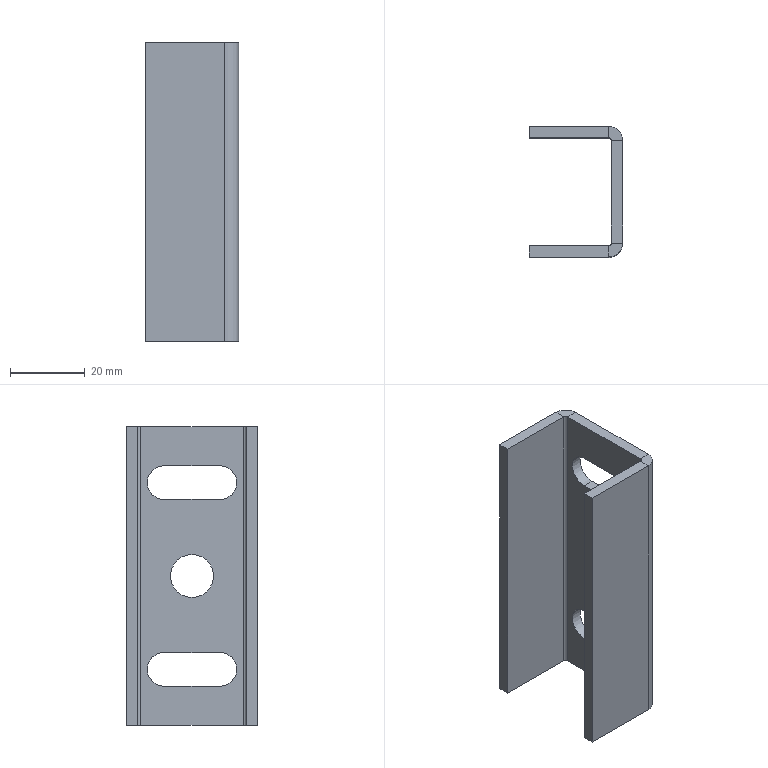Part | SolidWorks | features EdgeFlange 1, FlatPattern 1, SMBaseFlange 1, SheetMetal 1 | 1 solid | 32 faces | box 25 x 35 x 80 mm | volume 16996 mm3 | plane 22 | cylinder 10 | commonest cylinder face diameters 9 x4 1.473 x2 7.473 x2 11.5 x2
STEP:
#1=CARTESIAN_POINT('',(-3.,-17.5,-34.25));
#2=VERTEX_POINT('',#1);
#3=CARTESIAN_POINT('',(-3.,-17.5,-45.75));
#4=VERTEX_POINT('',#3);
#5=CARTESIAN_POINT('',(-3.,-17.5,-40.));
#6=DIRECTION('',(1.,0.,0.));
#7=DIRECTION('',(0.,0.,-1.));
#8=AXIS2_PLACEMENT_3D('',#5,#6,#7);
#9=CIRCLE('',#8,5.75);
#10=EDGE_CURVE('',#2,#4,#9,.T.);
#11=ORIENTED_EDGE('',*,*,#10,.F.);
#12=CARTESIAN_POINT('',(0.,-17.5,-34.25));
#13=VERTEX_POINT('',#12);
#14=CARTESIAN_POINT('',(-3.,-17.5,-34.25));
#15=DIRECTION('',(1.,0.,0.));
#16=VECTOR('',#15,1000.);
#17=LINE('',#14,#16);
#18=EDGE_CURVE('',#2,#13,#17,.T.);
#19=ORIENTED_EDGE('',*,*,#18,.T.);
#20=CARTESIAN_POINT('',(0.,-17.5,-45.75));
#21=VERTEX_POINT('',#20);
#22=CARTESIAN_POINT('',(0.,-17.5,-40.));
#23=DIRECTION('',(1.,0.,0.));
#24=DIRECTION('',(0.,0.,-1.));
#25=AXIS2_PLACEMENT_3D('',#22,#23,#24);
#26=CIRCLE('',#25,5.75);
#27=EDGE_CURVE('',#13,#21,#26,.T.);
#28=ORIENTED_EDGE('',*,*,#27,.T.);
#29=CARTESIAN_POINT('',(-3.,-17.5,-45.75));
#30=DIRECTION('',(1.,0.,0.));
#31=VECTOR('',#30,1000.);
#32=LINE('',#29,#31);
#33=EDGE_CURVE('',#4,#21,#32,.T.);
#34=ORIENTED_EDGE('',*,*,#33,.F.);
#35=EDGE_LOOP('',(#11,#19,#28,#34));
#36=FACE_OUTER_BOUND('',#35,.T.);
#37=CARTESIAN_POINT('',(-3.,-17.5,-40.));
#38=DIRECTION('',(1.,0.,0.));
#39=DIRECTION('',(0.,0.,-1.));
#40=AXIS2_PLACEMENT_3D('',#37,#38,#39);
#41=CYLINDRICAL_SURFACE('',#40,5.75);
#42=ADVANCED_FACE('',(#36),#41,.F.);
#43=CARTESIAN_POINT('',(-3.,-25.,-69.5));
#44=VERTEX_POINT('',#43);
#45=CARTESIAN_POINT('',(-3.,-10.,-69.5));
#46=VERTEX_POINT('',#45);
#47=CARTESIAN_POINT('',(-3.,-10.,-69.5));
#48=DIRECTION('',(0.,1.,0.));
#49=VECTOR('',#48,1000.);
#50=LINE('',#47,#49);
#51=EDGE_CURVE('',#44,#46,#50,.T.);
#52=ORIENTED_EDGE('',*,*,#51,.T.);
#53=CARTESIAN_POINT('',(-3.,-10.,-60.5));
#54=VERTEX_POINT('',#53);
#55=CARTESIAN_POINT('',(-3.,-10.,-65.));
#56=DIRECTION('',(1.,0.,0.));
#57=DIRECTION('',(0.,0.,-1.));
#58=AXIS2_PLACEMENT_3D('',#55,#56,#57);
#59=CIRCLE('',#58,4.5);
#60=EDGE_CURVE('',#46,#54,#59,.T.);
#61=ORIENTED_EDGE('',*,*,#60,.T.);
#62=CARTESIAN_POINT('',(-3.,-25.,-60.5));
#63=VERTEX_POINT('',#62);
#64=CARTESIAN_POINT('',(-3.,-10.,-60.5));
#65=DIRECTION('',(0.,-1.,0.));
#66=VECTOR('',#65,1000.);
#67=LINE('',#64,#66);
#68=EDGE_CURVE('',#54,#63,#67,.T.);
#69=ORIENTED_EDGE('',*,*,#68,.T.);
#70=CARTESIAN_POINT('',(-3.,-25.,-65.));
#71=DIRECTION('',(1.,0.,0.));
#72=DIRECTION('',(0.,0.,-1.));
#73=AXIS2_PLACEMENT_3D('',#70,#71,#72);
#74=CIRCLE('',#73,4.5);
#75=EDGE_CURVE('',#63,#44,#74,.T.);
#76=ORIENTED_EDGE('',*,*,#75,.T.);
#77=EDGE_LOOP('',(#52,#61,#69,#76));
#78=FACE_BOUND('',#77,.T.);
#79=CARTESIAN_POINT('',(-3.,-25.,-19.5));
#80=VERTEX_POINT('',#79);
#81=CARTESIAN_POINT('',(-3.,-10.,-19.5));
#82=VERTEX_POINT('',#81);
#83=CARTESIAN_POINT('',(-3.,-10.,-19.5));
#84=DIRECTION('',(0.,1.,0.));
#85=VECTOR('',#84,1000.);
#86=LINE('',#83,#85);
#87=EDGE_CURVE('',#80,#82,#86,.T.);
#88=ORIENTED_EDGE('',*,*,#87,.T.);
#89=CARTESIAN_POINT('',(-3.,-10.,-10.5));
#90=VERTEX_POINT('',#89);
#91=CARTESIAN_POINT('',(-3.,-10.,-15.));
#92=DIRECTION('',(1.,0.,0.));
#93=DIRECTION('',(0.,0.,-1.));
#94=AXIS2_PLACEMENT_3D('',#91,#92,#93);
#95=CIRCLE('',#94,4.5);
#96=EDGE_CURVE('',#82,#90,#95,.T.);
#97=ORIENTED_EDGE('',*,*,#96,.T.);
#98=CARTESIAN_POINT('',(-3.,-25.,-10.5));
#99=VERTEX_POINT('',#98);
#100=CARTESIAN_POINT('',(-3.,-10.,-10.5));
#101=DIRECTION('',(0.,-1.,0.));
#102=VECTOR('',#101,1000.);
#103=LINE('',#100,#102);
#104=EDGE_CURVE('',#90,#99,#103,.T.);
#105=ORIENTED_EDGE('',*,*,#104,.T.);
#106=CARTESIAN_POINT('',(-3.,-25.,-15.));
#107=DIRECTION('',(1.,0.,0.));
#108=DIRECTION('',(0.,0.,-1.));
#109=AXIS2_PLACEMENT_3D('',#106,#107,#108);
#110=CIRCLE('',#109,4.5);
#111=EDGE_CURVE('',#99,#80,#110,.T.);
#112=ORIENTED_EDGE('',*,*,#111,.T.);
#113=EDGE_LOOP('',(#88,#97,#105,#112));
#114=FACE_BOUND('',#113,.T.);
#115=CARTESIAN_POINT('',(-3.,-17.5,-40.));
#116=DIRECTION('',(1.,0.,0.));
#117=DIRECTION('',(0.,0.,-1.));
#118=AXIS2_PLACEMENT_3D('',#115,#116,#117);
#119=CIRCLE('',#118,5.75);
#120=EDGE_CURVE('',#4,#2,#119,.T.);
#121=ORIENTED_EDGE('',*,*,#120,.T.);
#122=ORIENTED_EDGE('',*,*,#10,.T.);
#123=EDGE_LOOP('',(#121,#122));
#124=FACE_BOUND('',#123,.T.);
#125=CARTESIAN_POINT('',(-3.,-31.263,0.));
#126=VERTEX_POINT('',#125);
#127=CARTESIAN_POINT('',(-3.,-31.263,-80.));
#128=VERTEX_POINT('',#127);
#129=CARTESIAN_POINT('',(-3.,-31.263,0.));
#130=DIRECTION('',(0.,0.,-1.));
#131=VECTOR('',#130,1000.);
#132=LINE('',#129,#131);
#133=EDGE_CURVE('',#126,#128,#132,.T.);
#134=ORIENTED_EDGE('',*,*,#133,.F.);
#135=CARTESIAN_POINT('',(-3.,-3.737,0.));
#136=VERTEX_POINT('',#135);
#137=CARTESIAN_POINT('',(-3.,0.,0.));
#138=DIRECTION('',(0.,-1.,0.));
#139=VECTOR('',#138,1000.);
#140=LINE('',#137,#139);
#141=EDGE_CURVE('',#136,#126,#140,.T.);
#142=ORIENTED_EDGE('',*,*,#141,.F.);
#143=CARTESIAN_POINT('',(-3.,-3.737,-80.));
#144=VERTEX_POINT('',#143);
#145=CARTESIAN_POINT('',(-3.,-3.737,-80.));
#146=DIRECTION('',(0.,0.,1.));
#147=VECTOR('',#146,1000.);
#148=LINE('',#145,#147);
#149=EDGE_CURVE('',#144,#136,#148,.T.);
#150=ORIENTED_EDGE('',*,*,#149,.F.);
#151=CARTESIAN_POINT('',(-3.,0.,-80.));
#152=DIRECTION('',(0.,1.,0.));
#153=VECTOR('',#152,1000.);
#154=LINE('',#151,#153);
#155=EDGE_CURVE('',#128,#144,#154,.T.);
#156=ORIENTED_EDGE('',*,*,#155,.F.);
#157=EDGE_LOOP('',(#134,#142,#150,#156));
#158=FACE_OUTER_BOUND('',#157,.T.);
#159=CARTESIAN_POINT('',(-3.,0.,0.));
#160=DIRECTION('',(1.,0.,0.));
#161=DIRECTION('',(0.,0.,-1.));
#162=AXIS2_PLACEMENT_3D('',#159,#160,#161);
#163=PLANE('',#162);
#164=ADVANCED_FACE('',(#78,#114,#124,#158),#163,.F.);
#165=CARTESIAN_POINT('',(0.,-10.,-69.5));
#166=VERTEX_POINT('',#165);
#167=CARTESIAN_POINT('',(0.,-10.,-60.5));
#168=VERTEX_POINT('',#167);
#169=CARTESIAN_POINT('',(0.,-10.,-65.));
#170=DIRECTION('',(1.,0.,0.));
#171=DIRECTION('',(0.,0.,-1.));
#172=AXIS2_PLACEMENT_3D('',#169,#170,#171);
#173=CIRCLE('',#172,4.5);
#174=EDGE_CURVE('',#166,#168,#173,.T.);
#175=ORIENTED_EDGE('',*,*,#174,.F.);
#176=CARTESIAN_POINT('',(0.,-25.,-69.5));
#177=VERTEX_POINT('',#176);
#178=CARTESIAN_POINT('',(0.,-10.,-69.5));
#179=DIRECTION('',(0.,1.,0.));
#180=VECTOR('',#179,1000.);
#181=LINE('',#178,#180);
#182=EDGE_CURVE('',#177,#166,#181,.T.);
#183=ORIENTED_EDGE('',*,*,#182,.F.);
#184=CARTESIAN_POINT('',(0.,-25.,-60.5));
#185=VERTEX_POINT('',#184);
#186=CARTESIAN_POINT('',(0.,-25.,-65.));
#187=DIRECTION('',(1.,0.,0.));
#188=DIRECTION('',(0.,0.,-1.));
#189=AXIS2_PLACEMENT_3D('',#186,#187,#188);
#190=CIRCLE('',#189,4.5);
#191=EDGE_CURVE('',#185,#177,#190,.T.);
#192=ORIENTED_EDGE('',*,*,#191,.F.);
#193=CARTESIAN_POINT('',(0.,-10.,-60.5));
#194=DIRECTION('',(0.,-1.,0.));
#195=VECTOR('',#194,1000.);
#196=LINE('',#193,#195);
#197=EDGE_CURVE('',#168,#185,#196,.T.);
#198=ORIENTED_EDGE('',*,*,#197,.F.);
#199=EDGE_LOOP('',(#175,#183,#192,#198));
#200=FACE_BOUND('',#199,.T.);
#201=CARTESIAN_POINT('',(0.,-10.,-19.5));
#202=VERTEX_POINT('',#201);
#203=CARTESIAN_POINT('',(0.,-10.,-10.5));
#204=VERTEX_POINT('',#203);
#205=CARTESIAN_POINT('',(0.,-10.,-15.));
#206=DIRECTION('',(1.,0.,0.));
#207=DIRECTION('',(0.,0.,-1.));
#208=AXIS2_PLACEMENT_3D('',#205,#206,#207);
#209=CIRCLE('',#208,4.5);
#210=EDGE_CURVE('',#202,#204,#209,.T.);
#211=ORIENTED_EDGE('',*,*,#210,.F.);
#212=CARTESIAN_POINT('',(0.,-25.,-19.5));
#213=VERTEX_POINT('',#212);
#214=CARTESIAN_POINT('',(0.,-10.,-19.5));
#215=DIRECTION('',(0.,1.,0.));
#216=VECTOR('',#215,1000.);
#217=LINE('',#214,#216);
#218=EDGE_CURVE('',#213,#202,#217,.T.);
#219=ORIENTED_EDGE('',*,*,#218,.F.);
#220=CARTESIAN_POINT('',(0.,-25.,-10.5));
#221=VERTEX_POINT('',#220);
#222=CARTESIAN_POINT('',(0.,-25.,-15.));
#223=DIRECTION('',(1.,0.,0.));
#224=DIRECTION('',(0.,0.,-1.));
#225=AXIS2_PLACEMENT_3D('',#222,#223,#224);
#226=CIRCLE('',#225,4.5);
#227=EDGE_CURVE('',#221,#213,#226,.T.);
#228=ORIENTED_EDGE('',*,*,#227,.F.);
#229=CARTESIAN_POINT('',(0.,-10.,-10.5));
#230=DIRECTION('',(0.,-1.,0.));
#231=VECTOR('',#230,1000.);
#232=LINE('',#229,#231);
#233=EDGE_CURVE('',#204,#221,#232,.T.);
#234=ORIENTED_EDGE('',*,*,#233,.F.);
#235=EDGE_LOOP('',(#211,#219,#228,#234));
#236=FACE_BOUND('',#235,.T.);
#237=CARTESIAN_POINT('',(0.,-17.5,-40.));
#238=DIRECTION('',(1.,0.,0.));
#239=DIRECTION('',(0.,0.,-1.));
#240=AXIS2_PLACEMENT_3D('',#237,#238,#239);
#241=CIRCLE('',#240,5.75);
#242=EDGE_CURVE('',#21,#13,#241,.T.);
#243=ORIENTED_EDGE('',*,*,#242,.F.);
#244=ORIENTED_EDGE('',*,*,#27,.F.);
#245=EDGE_LOOP('',(#243,#244));
#246=FACE_BOUND('',#245,.T.);
#247=CARTESIAN_POINT('',(0.,-3.737,0.));
#248=VERTEX_POINT('',#247);
#249=CARTESIAN_POINT('',(0.,-31.263,0.));
#250=VERTEX_POINT('',#249);
#251=CARTESIAN_POINT('',(0.,0.,0.));
#252=DIRECTION('',(0.,-1.,0.));
#253=VECTOR('',#252,1000.);
#254=LINE('',#251,#253);
#255=EDGE_CURVE('',#248,#250,#254,.T.);
#256=ORIENTED_EDGE('',*,*,#255,.T.);
#257=CARTESIAN_POINT('',(0.,-31.263,-80.));
#258=VERTEX_POINT('',#257);
#259=CARTESIAN_POINT('',(0.,-31.263,0.));
#260=DIRECTION('',(0.,0.,-1.));
#261=VECTOR('',#260,1000.);
#262=LINE('',#259,#261);
#263=EDGE_CURVE('',#250,#258,#262,.T.);
#264=ORIENTED_EDGE('',*,*,#263,.T.);
#265=CARTESIAN_POINT('',(0.,-3.737,-80.));
#266=VERTEX_POINT('',#265);
#267=CARTESIAN_POINT('',(0.,0.,-80.));
#268=DIRECTION('',(0.,1.,0.));
#269=VECTOR('',#268,1000.);
#270=LINE('',#267,#269);
#271=EDGE_CURVE('',#258,#266,#270,.T.);
#272=ORIENTED_EDGE('',*,*,#271,.T.);
#273=CARTESIAN_POINT('',(0.,-3.737,-80.));
#274=DIRECTION('',(0.,0.,1.));
#275=VECTOR('',#274,1000.);
#276=LINE('',#273,#275);
#277=EDGE_CURVE('',#266,#248,#276,.T.);
#278=ORIENTED_EDGE('',*,*,#277,.T.);
#279=EDGE_LOOP('',(#256,#264,#272,#278));
#280=FACE_OUTER_BOUND('',#279,.T.);
#281=CARTESIAN_POINT('',(0.,0.,0.));
#282=DIRECTION('',(1.,0.,0.));
#283=DIRECTION('',(0.,0.,-1.));
#284=AXIS2_PLACEMENT_3D('',#281,#282,#283);
#285=PLANE('',#284);
#286=ADVANCED_FACE('',(#200,#236,#246,#280),#285,.T.);
#287=ORIENTED_EDGE('',*,*,#141,.T.);
#288=CARTESIAN_POINT('',(-3.,-31.263,0.));
#289=DIRECTION('',(1.,0.,0.));
#290=VECTOR('',#289,1000.);
#291=LINE('',#288,#290);
#292=EDGE_CURVE('',#126,#250,#291,.T.);
#293=ORIENTED_EDGE('',*,*,#292,.T.);
#294=ORIENTED_EDGE('',*,*,#255,.F.);
#295=CARTESIAN_POINT('',(-3.,-3.737,0.));
#296=DIRECTION('',(1.,0.,0.));
#297=VECTOR('',#296,1000.);
#298=LINE('',#295,#297);
#299=EDGE_CURVE('',#136,#248,#298,.T.);
#300=ORIENTED_EDGE('',*,*,#299,.F.);
#301=EDGE_LOOP('',(#287,#293,#294,#300));
#302=FACE_OUTER_BOUND('',#301,.T.);
#303=CARTESIAN_POINT('',(-3.,0.,0.));
#304=DIRECTION('',(0.,0.,1.));
#305=DIRECTION('',(0.,-1.,0.));
#306=AXIS2_PLACEMENT_3D('',#303,#304,#305);
#307=PLANE('',#306);
#308=ADVANCED_FACE('',(#302),#307,.T.);
#309=CARTESIAN_POINT('',(-3.,-31.263,-80.));
#310=DIRECTION('',(1.,0.,0.));
#311=VECTOR('',#310,1000.);
#312=LINE('',#309,#311);
#313=EDGE_CURVE('',#128,#258,#312,.T.);
#314=ORIENTED_EDGE('',*,*,#313,.F.);
#315=ORIENTED_EDGE('',*,*,#155,.T.);
#316=CARTESIAN_POINT('',(-3.,-3.737,-80.));
#317=DIRECTION('',(1.,0.,0.));
#318=VECTOR('',#317,1000.);
#319=LINE('',#316,#318);
#320=EDGE_CURVE('',#144,#266,#319,.T.);
#321=ORIENTED_EDGE('',*,*,#320,.T.);
#322=ORIENTED_EDGE('',*,*,#271,.F.);
#323=EDGE_LOOP('',(#314,#315,#321,#322));
#324=FACE_OUTER_BOUND('',#323,.T.);
#325=CARTESIAN_POINT('',(-3.,0.,-80.));
#326=DIRECTION('',(0.,0.,-1.));
#327=DIRECTION('',(-1.,0.,0.));
#328=AXIS2_PLACEMENT_3D('',#325,#326,#327);
#329=PLANE('',#328);
#330=ADVANCED_FACE('',(#324),#329,.T.);
#331=ORIENTED_EDGE('',*,*,#18,.F.);
#332=ORIENTED_EDGE('',*,*,#120,.F.);
#333=ORIENTED_EDGE('',*,*,#33,.T.);
#334=ORIENTED_EDGE('',*,*,#242,.T.);
#335=EDGE_LOOP('',(#331,#332,#333,#334));
#336=FACE_OUTER_BOUND('',#335,.T.);
#337=CARTESIAN_POINT('',(-3.,-17.5,-40.));
#338=DIRECTION('',(1.,0.,0.));
#339=DIRECTION('',(0.,0.,-1.));
#340=AXIS2_PLACEMENT_3D('',#337,#338,#339);
#341=CYLINDRICAL_SURFACE('',#340,5.75);
#342=ADVANCED_FACE('',(#336),#341,.F.);
#343=ORIENTED_EDGE('',*,*,#210,.T.);
#344=CARTESIAN_POINT('',(-3.,-10.,-10.5));
#345=DIRECTION('',(1.,0.,0.));
#346=VECTOR('',#345,1000.);
#347=LINE('',#344,#346);
#348=EDGE_CURVE('',#90,#204,#347,.T.);
#349=ORIENTED_EDGE('',*,*,#348,.F.);
#350=ORIENTED_EDGE('',*,*,#96,.F.);
#351=CARTESIAN_POINT('',(-3.,-10.,-19.5));
#352=DIRECTION('',(1.,0.,0.));
#353=VECTOR('',#352,1000.);
#354=LINE('',#351,#353);
#355=EDGE_CURVE('',#82,#202,#354,.T.);
#356=ORIENTED_EDGE('',*,*,#355,.T.);
#357=EDGE_LOOP('',(#343,#349,#350,#356));
#358=FACE_OUTER_BOUND('',#357,.T.);
#359=CARTESIAN_POINT('',(-3.,-10.,-15.));
#360=DIRECTION('',(1.,0.,0.));
#361=DIRECTION('',(0.,0.,-1.));
#362=AXIS2_PLACEMENT_3D('',#359,#360,#361);
#363=CYLINDRICAL_SURFACE('',#362,4.5);
#364=ADVANCED_FACE('',(#358),#363,.F.);
#365=ORIENTED_EDGE('',*,*,#218,.T.);
#366=ORIENTED_EDGE('',*,*,#355,.F.);
#367=ORIENTED_EDGE('',*,*,#87,.F.);
#368=CARTESIAN_POINT('',(-3.,-25.,-19.5));
#369=DIRECTION('',(1.,0.,0.));
#370=VECTOR('',#369,1000.);
#371=LINE('',#368,#370);
#372=EDGE_CURVE('',#80,#213,#371,.T.);
#373=ORIENTED_EDGE('',*,*,#372,.T.);
#374=EDGE_LOOP('',(#365,#366,#367,#373));
#375=FACE_OUTER_BOUND('',#374,.T.);
#376=CARTESIAN_POINT('',(-3.,-10.,-19.5));
#377=DIRECTION('',(0.,0.,-1.));
#378=DIRECTION('',(0.,1.,0.));
#379=AXIS2_PLACEMENT_3D('',#376,#377,#378);
#380=PLANE('',#379);
#381=ADVANCED_FACE('',(#375),#380,.F.);
#382=ORIENTED_EDGE('',*,*,#227,.T.);
#383=ORIENTED_EDGE('',*,*,#372,.F.);
#384=ORIENTED_EDGE('',*,*,#111,.F.);
#385=CARTESIAN_POINT('',(-3.,-25.,-10.5));
#386=DIRECTION('',(1.,0.,0.));
#387=VECTOR('',#386,1000.);
#388=LINE('',#385,#387);
#389=EDGE_CURVE('',#99,#221,#388,.T.);
#390=ORIENTED_EDGE('',*,*,#389,.T.);
#391=EDGE_LOOP('',(#382,#383,#384,#390));
#392=FACE_OUTER_BOUND('',#391,.T.);
#393=CARTESIAN_POINT('',(-3.,-25.,-15.));
#394=DIRECTION('',(1.,0.,0.));
#395=DIRECTION('',(0.,0.,-1.));
#396=AXIS2_PLACEMENT_3D('',#393,#394,#395);
#397=CYLINDRICAL_SURFACE('',#396,4.5);
#398=ADVANCED_FACE('',(#392),#397,.F.);
#399=ORIENTED_EDGE('',*,*,#233,.T.);
#400=ORIENTED_EDGE('',*,*,#389,.F.);
#401=ORIENTED_EDGE('',*,*,#104,.F.);
#402=ORIENTED_EDGE('',*,*,#348,.T.);
#403=EDGE_LOOP('',(#399,#400,#401,#402));
#404=FACE_OUTER_BOUND('',#403,.T.);
#405=CARTESIAN_POINT('',(-3.,-10.,-10.5));
#406=DIRECTION('',(0.,0.,1.));
#407=DIRECTION('',(0.,-1.,0.));
#408=AXIS2_PLACEMENT_3D('',#405,#406,#407);
#409=PLANE('',#408);
#410=ADVANCED_FACE('',(#404),#409,.F.);
#411=ORIENTED_EDGE('',*,*,#174,.T.);
#412=CARTESIAN_POINT('',(-3.,-10.,-60.5));
#413=DIRECTION('',(1.,0.,0.));
#414=VECTOR('',#413,1000.);
#415=LINE('',#412,#414);
#416=EDGE_CURVE('',#54,#168,#415,.T.);
#417=ORIENTED_EDGE('',*,*,#416,.F.);
#418=ORIENTED_EDGE('',*,*,#60,.F.);
#419=CARTESIAN_POINT('',(-3.,-10.,-69.5));
#420=DIRECTION('',(1.,0.,0.));
#421=VECTOR('',#420,1000.);
#422=LINE('',#419,#421);
#423=EDGE_CURVE('',#46,#166,#422,.T.);
#424=ORIENTED_EDGE('',*,*,#423,.T.);
#425=EDGE_LOOP('',(#411,#417,#418,#424));
#426=FACE_OUTER_BOUND('',#425,.T.);
#427=CARTESIAN_POINT('',(-3.,-10.,-65.));
#428=DIRECTION('',(1.,0.,0.));
#429=DIRECTION('',(0.,0.,-1.));
#430=AXIS2_PLACEMENT_3D('',#427,#428,#429);
#431=CYLINDRICAL_SURFACE('',#430,4.5);
#432=ADVANCED_FACE('',(#426),#431,.F.);
#433=ORIENTED_EDGE('',*,*,#182,.T.);
#434=ORIENTED_EDGE('',*,*,#423,.F.);
#435=ORIENTED_EDGE('',*,*,#51,.F.);
#436=CARTESIAN_POINT('',(-3.,-25.,-69.5));
#437=DIRECTION('',(1.,0.,0.));
#438=VECTOR('',#437,1000.);
#439=LINE('',#436,#438);
#440=EDGE_CURVE('',#44,#177,#439,.T.);
#441=ORIENTED_EDGE('',*,*,#440,.T.);
#442=EDGE_LOOP('',(#433,#434,#435,#441));
#443=FACE_OUTER_BOUND('',#442,.T.);
#444=CARTESIAN_POINT('',(-3.,-10.,-69.5));
#445=DIRECTION('',(0.,0.,-1.));
#446=DIRECTION('',(0.,1.,0.));
#447=AXIS2_PLACEMENT_3D('',#444,#445,#446);
#448=PLANE('',#447);
#449=ADVANCED_FACE('',(#443),#448,.F.);
#450=ORIENTED_EDGE('',*,*,#191,.T.);
#451=ORIENTED_EDGE('',*,*,#440,.F.);
#452=ORIENTED_EDGE('',*,*,#75,.F.);
#453=CARTESIAN_POINT('',(-3.,-25.,-60.5));
#454=DIRECTION('',(1.,0.,0.));
#455=VECTOR('',#454,1000.);
#456=LINE('',#453,#455);
#457=EDGE_CURVE('',#63,#185,#456,.T.);
#458=ORIENTED_EDGE('',*,*,#457,.T.);
#459=EDGE_LOOP('',(#450,#451,#452,#458));
#460=FACE_OUTER_BOUND('',#459,.T.);
#461=CARTESIAN_POINT('',(-3.,-25.,-65.));
#462=DIRECTION('',(1.,0.,0.));
#463=DIRECTION('',(0.,0.,-1.));
#464=AXIS2_PLACEMENT_3D('',#461,#462,#463);
#465=CYLINDRICAL_SURFACE('',#464,4.5);
#466=ADVANCED_FACE('',(#460),#465,.F.);
#467=ORIENTED_EDGE('',*,*,#197,.T.);
#468=ORIENTED_EDGE('',*,*,#457,.F.);
#469=ORIENTED_EDGE('',*,*,#68,.F.);
#470=ORIENTED_EDGE('',*,*,#416,.T.);
#471=EDGE_LOOP('',(#467,#468,#469,#470));
#472=FACE_OUTER_BOUND('',#471,.T.);
#473=CARTESIAN_POINT('',(-3.,-10.,-60.5));
#474=DIRECTION('',(0.,0.,1.));
#475=DIRECTION('',(0.,-1.,0.));
#476=AXIS2_PLACEMENT_3D('',#473,#474,#475);
#477=PLANE('',#476);
#478=ADVANCED_FACE('',(#472),#477,.F.);
#479=CARTESIAN_POINT('',(-3.737,-3.,0.));
#480=VERTEX_POINT('',#479);
#481=CARTESIAN_POINT('',(-3.737,0.,0.));
#482=VERTEX_POINT('',#481);
#483=CARTESIAN_POINT('',(-3.737,0.,0.));
#484=DIRECTION('',(0.,1.,0.));
#485=VECTOR('',#484,1000.);
#486=LINE('',#483,#485);
#487=EDGE_CURVE('',#480,#482,#486,.T.);
#488=ORIENTED_EDGE('',*,*,#487,.F.);
#489=CARTESIAN_POINT('',(-3.737,-3.737,0.));
#490=DIRECTION('',(0.,0.,1.));
#491=DIRECTION('',(-1.,0.,0.));
#492=AXIS2_PLACEMENT_3D('',#489,#490,#491);
#493=CIRCLE('',#492,0.7366);
#494=EDGE_CURVE('',#136,#480,#493,.T.);
#495=ORIENTED_EDGE('',*,*,#494,.F.);
#496=ORIENTED_EDGE('',*,*,#299,.T.);
#497=CARTESIAN_POINT('',(-3.737,-3.737,0.));
#498=DIRECTION('',(0.,0.,1.));
#499=DIRECTION('',(-1.,0.,0.));
#500=AXIS2_PLACEMENT_3D('',#497,#498,#499);
#501=CIRCLE('',#500,3.737);
#502=EDGE_CURVE('',#248,#482,#501,.T.);
#503=ORIENTED_EDGE('',*,*,#502,.T.);
#504=EDGE_LOOP('',(#488,#495,#496,#503));
#505=FACE_OUTER_BOUND('',#504,.T.);
#506=CARTESIAN_POINT('',(-3.737,-3.737,0.));
#507=DIRECTION('',(0.,0.,1.));
#508=DIRECTION('',(1.,0.,0.));
#509=AXIS2_PLACEMENT_3D('',#506,#507,#508);
#510=PLANE('',#509);
#511=ADVANCED_FACE('',(#505),#510,.T.);
#512=CARTESIAN_POINT('',(-3.737,-3.,-80.));
#513=VERTEX_POINT('',#512);
#514=CARTESIAN_POINT('',(-3.737,-3.737,-80.));
#515=DIRECTION('',(0.,0.,-1.));
#516=DIRECTION('',(-1.,0.,0.));
#517=AXIS2_PLACEMENT_3D('',#514,#515,#516);
#518=CIRCLE('',#517,0.7366);
#519=EDGE_CURVE('',#513,#144,#518,.T.);
#520=ORIENTED_EDGE('',*,*,#519,.F.);
#521=CARTESIAN_POINT('',(-3.737,0.,-80.));
#522=VERTEX_POINT('',#521);
#523=CARTESIAN_POINT('',(-3.737,-3.,-80.));
#524=DIRECTION('',(0.,1.,0.));
#525=VECTOR('',#524,1000.);
#526=LINE('',#523,#525);
#527=EDGE_CURVE('',#513,#522,#526,.T.);
#528=ORIENTED_EDGE('',*,*,#527,.T.);
#529=CARTESIAN_POINT('',(-3.737,-3.737,-80.));
#530=DIRECTION('',(0.,0.,-1.));
#531=DIRECTION('',(-1.,0.,0.));
#532=AXIS2_PLACEMENT_3D('',#529,#530,#531);
#533=CIRCLE('',#532,3.737);
#534=EDGE_CURVE('',#522,#266,#533,.T.);
#535=ORIENTED_EDGE('',*,*,#534,.T.);
#536=ORIENTED_EDGE('',*,*,#320,.F.);
#537=EDGE_LOOP('',(#520,#528,#535,#536));
#538=FACE_OUTER_BOUND('',#537,.T.);
#539=CARTESIAN_POINT('',(-3.737,-3.737,-80.));
#540=DIRECTION('',(0.,0.,1.));
#541=DIRECTION('',(1.,0.,0.));
#542=AXIS2_PLACEMENT_3D('',#539,#540,#541);
#543=PLANE('',#542);
#544=ADVANCED_FACE('',(#538),#543,.F.);
#545=ORIENTED_EDGE('',*,*,#277,.F.);
#546=ORIENTED_EDGE('',*,*,#534,.F.);
#547=CARTESIAN_POINT('',(-3.737,0.,0.));
#548=DIRECTION('',(0.,0.,1.));
#549=VECTOR('',#548,1000.);
#550=LINE('',#547,#549);
#551=EDGE_CURVE('',#522,#482,#550,.T.);
#552=ORIENTED_EDGE('',*,*,#551,.T.);
#553=ORIENTED_EDGE('',*,*,#502,.F.);
#554=EDGE_LOOP('',(#545,#546,#552,#553));
#555=FACE_OUTER_BOUND('',#554,.T.);
#556=CARTESIAN_POINT('',(-3.737,-3.737,-80.));
#557=DIRECTION('',(0.,0.,-1.));
#558=DIRECTION('',(0.,1.,0.));
#559=AXIS2_PLACEMENT_3D('',#556,#557,#558);
#560=CYLINDRICAL_SURFACE('',#559,3.737);
#561=ADVANCED_FACE('',(#555),#560,.T.);
#562=ORIENTED_EDGE('',*,*,#149,.T.);
#563=ORIENTED_EDGE('',*,*,#494,.T.);
#564=CARTESIAN_POINT('',(-3.737,-3.,0.));
#565=DIRECTION('',(0.,0.,-1.));
#566=VECTOR('',#565,1000.);
#567=LINE('',#564,#566);
#568=EDGE_CURVE('',#480,#513,#567,.T.);
#569=ORIENTED_EDGE('',*,*,#568,.T.);
#570=ORIENTED_EDGE('',*,*,#519,.T.);
#571=EDGE_LOOP('',(#562,#563,#569,#570));
#572=FACE_OUTER_BOUND('',#571,.T.);
#573=CARTESIAN_POINT('',(-3.737,-3.737,-80.));
#574=DIRECTION('',(0.,0.,-1.));
#575=DIRECTION('',(0.,1.,0.));
#576=AXIS2_PLACEMENT_3D('',#573,#574,#575);
#577=CYLINDRICAL_SURFACE('',#576,0.7366);
#578=ADVANCED_FACE('',(#572),#577,.F.);
#579=ORIENTED_EDGE('',*,*,#527,.F.);
#580=CARTESIAN_POINT('',(-25.,-3.,-80.));
#581=VERTEX_POINT('',#580);
#582=CARTESIAN_POINT('',(-25.,-3.,-80.));
#583=DIRECTION('',(-1.,0.,0.));
#584=VECTOR('',#583,1000.);
#585=LINE('',#582,#584);
#586=EDGE_CURVE('',#513,#581,#585,.T.);
#587=ORIENTED_EDGE('',*,*,#586,.T.);
#588=CARTESIAN_POINT('',(-25.,0.,-80.));
#589=VERTEX_POINT('',#588);
#590=CARTESIAN_POINT('',(-25.,0.,-80.));
#591=DIRECTION('',(0.,-1.,0.));
#592=VECTOR('',#591,1000.);
#593=LINE('',#590,#592);
#594=EDGE_CURVE('',#589,#581,#593,.T.);
#595=ORIENTED_EDGE('',*,*,#594,.F.);
#596=CARTESIAN_POINT('',(0.,0.,-80.));
#597=DIRECTION('',(-1.,0.,0.));
#598=VECTOR('',#597,1000.);
#599=LINE('',#596,#598);
#600=EDGE_CURVE('',#522,#589,#599,.T.);
#601=ORIENTED_EDGE('',*,*,#600,.F.);
#602=EDGE_LOOP('',(#579,#587,#595,#601));
#603=FACE_OUTER_BOUND('',#602,.T.);
#604=CARTESIAN_POINT('',(-25.,0.,-80.));
#605=DIRECTION('',(0.,0.,1.));
#606=DIRECTION('',(1.,0.,0.));
#607=AXIS2_PLACEMENT_3D('',#604,#605,#606);
#608=PLANE('',#607);
#609=ADVANCED_FACE('',(#603),#608,.F.);
#610=ORIENTED_EDGE('',*,*,#487,.T.);
#611=CARTESIAN_POINT('',(-25.,0.,0.));
#612=VERTEX_POINT('',#611);
#613=CARTESIAN_POINT('',(0.,0.,0.));
#614=DIRECTION('',(1.,0.,0.));
#615=VECTOR('',#614,1000.);
#616=LINE('',#613,#615);
#617=EDGE_CURVE('',#612,#482,#616,.T.);
#618=ORIENTED_EDGE('',*,*,#617,.F.);
#619=CARTESIAN_POINT('',(-25.,-3.,0.));
#620=VERTEX_POINT('',#619);
#621=CARTESIAN_POINT('',(-25.,0.,0.));
#622=DIRECTION('',(0.,-1.,0.));
#623=VECTOR('',#622,1000.);
#624=LINE('',#621,#623);
#625=EDGE_CURVE('',#612,#620,#624,.T.);
#626=ORIENTED_EDGE('',*,*,#625,.T.);
#627=CARTESIAN_POINT('',(-3.,-3.,0.));
#628=DIRECTION('',(1.,0.,0.));
#629=VECTOR('',#628,1000.);
#630=LINE('',#627,#629);
#631=EDGE_CURVE('',#620,#480,#630,.T.);
#632=ORIENTED_EDGE('',*,*,#631,.T.);
#633=EDGE_LOOP('',(#610,#618,#626,#632));
#634=FACE_OUTER_BOUND('',#633,.T.);
#635=CARTESIAN_POINT('',(-3.,0.,0.));
#636=DIRECTION('',(0.,0.,-1.));
#637=DIRECTION('',(-1.,0.,0.));
#638=AXIS2_PLACEMENT_3D('',#635,#636,#637);
#639=PLANE('',#638);
#640=ADVANCED_FACE('',(#634),#639,.F.);
#641=ORIENTED_EDGE('',*,*,#551,.F.);
#642=ORIENTED_EDGE('',*,*,#600,.T.);
#643=CARTESIAN_POINT('',(-25.,0.,0.));
#644=DIRECTION('',(0.,0.,1.));
#645=VECTOR('',#644,1000.);
#646=LINE('',#643,#645);
#647=EDGE_CURVE('',#589,#612,#646,.T.);
#648=ORIENTED_EDGE('',*,*,#647,.T.);
#649=ORIENTED_EDGE('',*,*,#617,.T.);
#650=EDGE_LOOP('',(#641,#642,#648,#649));
#651=FACE_OUTER_BOUND('',#650,.T.);
#652=CARTESIAN_POINT('',(0.,0.,0.));
#653=DIRECTION('',(0.,-1.,0.));
#654=DIRECTION('',(1.,0.,0.));
#655=AXIS2_PLACEMENT_3D('',#652,#653,#654);
#656=PLANE('',#655);
#657=ADVANCED_FACE('',(#651),#656,.F.);
#658=ORIENTED_EDGE('',*,*,#586,.F.);
#659=ORIENTED_EDGE('',*,*,#568,.F.);
#660=ORIENTED_EDGE('',*,*,#631,.F.);
#661=CARTESIAN_POINT('',(-25.,-3.,0.));
#662=DIRECTION('',(0.,0.,1.));
#663=VECTOR('',#662,1000.);
#664=LINE('',#661,#663);
#665=EDGE_CURVE('',#581,#620,#664,.T.);
#666=ORIENTED_EDGE('',*,*,#665,.F.);
#667=EDGE_LOOP('',(#658,#659,#660,#666));
#668=FACE_OUTER_BOUND('',#667,.T.);
#669=CARTESIAN_POINT('',(0.,-3.,0.));
#670=DIRECTION('',(0.,-1.,0.));
#671=DIRECTION('',(1.,0.,0.));
#672=AXIS2_PLACEMENT_3D('',#669,#670,#671);
#673=PLANE('',#672);
#674=ADVANCED_FACE('',(#668),#673,.T.);
#675=ORIENTED_EDGE('',*,*,#665,.T.);
#676=ORIENTED_EDGE('',*,*,#625,.F.);
#677=ORIENTED_EDGE('',*,*,#647,.F.);
#678=ORIENTED_EDGE('',*,*,#594,.T.);
#679=EDGE_LOOP('',(#675,#676,#677,#678));
#680=FACE_OUTER_BOUND('',#679,.T.);
#681=CARTESIAN_POINT('',(-25.,0.,0.));
#682=DIRECTION('',(1.,0.,0.));
#683=DIRECTION('',(0.,1.,0.));
#684=AXIS2_PLACEMENT_3D('',#681,#682,#683);
#685=PLANE('',#684);
#686=ADVANCED_FACE('',(#680),#685,.F.);
#687=CARTESIAN_POINT('',(-3.737,-32.,-80.));
#688=VERTEX_POINT('',#687);
#689=CARTESIAN_POINT('',(-3.737,-35.,-80.));
#690=VERTEX_POINT('',#689);
#691=CARTESIAN_POINT('',(-3.737,-35.,-80.));
#692=DIRECTION('',(0.,-1.,0.));
#693=VECTOR('',#692,1000.);
#694=LINE('',#691,#693);
#695=EDGE_CURVE('',#688,#690,#694,.T.);
#696=ORIENTED_EDGE('',*,*,#695,.F.);
#697=CARTESIAN_POINT('',(-3.737,-31.263,-80.));
#698=DIRECTION('',(0.,0.,-1.));
#699=DIRECTION('',(1.,0.,0.));
#700=AXIS2_PLACEMENT_3D('',#697,#698,#699);
#701=CIRCLE('',#700,0.7366);
#702=EDGE_CURVE('',#128,#688,#701,.T.);
#703=ORIENTED_EDGE('',*,*,#702,.F.);
#704=ORIENTED_EDGE('',*,*,#313,.T.);
#705=CARTESIAN_POINT('',(-3.737,-31.263,-80.));
#706=DIRECTION('',(0.,0.,-1.));
#707=DIRECTION('',(1.,0.,0.));
#708=AXIS2_PLACEMENT_3D('',#705,#706,#707);
#709=CIRCLE('',#708,3.737);
#710=EDGE_CURVE('',#258,#690,#709,.T.);
#711=ORIENTED_EDGE('',*,*,#710,.T.);
#712=EDGE_LOOP('',(#696,#703,#704,#711));
#713=FACE_OUTER_BOUND('',#712,.T.);
#714=CARTESIAN_POINT('',(-3.737,-31.263,-80.));
#715=DIRECTION('',(0.,0.,-1.));
#716=DIRECTION('',(-1.,0.,0.));
#717=AXIS2_PLACEMENT_3D('',#714,#715,#716);
#718=PLANE('',#717);
#719=ADVANCED_FACE('',(#713),#718,.T.);
#720=CARTESIAN_POINT('',(-3.737,-32.,0.));
#721=VERTEX_POINT('',#720);
#722=CARTESIAN_POINT('',(-3.737,-31.263,0.));
#723=DIRECTION('',(0.,0.,1.));
#724=DIRECTION('',(1.,0.,0.));
#725=AXIS2_PLACEMENT_3D('',#722,#723,#724);
#726=CIRCLE('',#725,0.7366);
#727=EDGE_CURVE('',#721,#126,#726,.T.);
#728=ORIENTED_EDGE('',*,*,#727,.F.);
#729=CARTESIAN_POINT('',(-3.737,-35.,0.));
#730=VERTEX_POINT('',#729);
#731=CARTESIAN_POINT('',(-3.737,-32.,0.));
#732=DIRECTION('',(0.,-1.,0.));
#733=VECTOR('',#732,1000.);
#734=LINE('',#731,#733);
#735=EDGE_CURVE('',#721,#730,#734,.T.);
#736=ORIENTED_EDGE('',*,*,#735,.T.);
#737=CARTESIAN_POINT('',(-3.737,-31.263,0.));
#738=DIRECTION('',(0.,0.,1.));
#739=DIRECTION('',(1.,0.,0.));
#740=AXIS2_PLACEMENT_3D('',#737,#738,#739);
#741=CIRCLE('',#740,3.737);
#742=EDGE_CURVE('',#730,#250,#741,.T.);
#743=ORIENTED_EDGE('',*,*,#742,.T.);
#744=ORIENTED_EDGE('',*,*,#292,.F.);
#745=EDGE_LOOP('',(#728,#736,#743,#744));
#746=FACE_OUTER_BOUND('',#745,.T.);
#747=CARTESIAN_POINT('',(-3.737,-31.263,0.));
#748=DIRECTION('',(0.,0.,-1.));
#749=DIRECTION('',(-1.,0.,0.));
#750=AXIS2_PLACEMENT_3D('',#747,#748,#749);
#751=PLANE('',#750);
#752=ADVANCED_FACE('',(#746),#751,.F.);
#753=ORIENTED_EDGE('',*,*,#263,.F.);
#754=ORIENTED_EDGE('',*,*,#742,.F.);
#755=CARTESIAN_POINT('',(-3.737,-35.,0.));
#756=DIRECTION('',(0.,0.,1.));
#757=VECTOR('',#756,1000.);
#758=LINE('',#755,#757);
#759=EDGE_CURVE('',#690,#730,#758,.T.);
#760=ORIENTED_EDGE('',*,*,#759,.F.);
#761=ORIENTED_EDGE('',*,*,#710,.F.);
#762=EDGE_LOOP('',(#753,#754,#760,#761));
#763=FACE_OUTER_BOUND('',#762,.T.);
#764=CARTESIAN_POINT('',(-3.737,-31.263,0.));
#765=DIRECTION('',(0.,0.,1.));
#766=DIRECTION('',(0.,-1.,0.));
#767=AXIS2_PLACEMENT_3D('',#764,#765,#766);
#768=CYLINDRICAL_SURFACE('',#767,3.737);
#769=ADVANCED_FACE('',(#763),#768,.T.);
#770=ORIENTED_EDGE('',*,*,#133,.T.);
#771=ORIENTED_EDGE('',*,*,#702,.T.);
#772=CARTESIAN_POINT('',(-3.737,-32.,-80.));
#773=DIRECTION('',(0.,0.,1.));
#774=VECTOR('',#773,1000.);
#775=LINE('',#772,#774);
#776=EDGE_CURVE('',#688,#721,#775,.T.);
#777=ORIENTED_EDGE('',*,*,#776,.T.);
#778=ORIENTED_EDGE('',*,*,#727,.T.);
#779=EDGE_LOOP('',(#770,#771,#777,#778));
#780=FACE_OUTER_BOUND('',#779,.T.);
#781=CARTESIAN_POINT('',(-3.737,-31.263,0.));
#782=DIRECTION('',(0.,0.,1.));
#783=DIRECTION('',(0.,-1.,0.));
#784=AXIS2_PLACEMENT_3D('',#781,#782,#783);
#785=CYLINDRICAL_SURFACE('',#784,0.7366);
#786=ADVANCED_FACE('',(#780),#785,.F.);
#787=ORIENTED_EDGE('',*,*,#735,.F.);
#788=CARTESIAN_POINT('',(-25.,-32.,0.));
#789=VERTEX_POINT('',#788);
#790=CARTESIAN_POINT('',(-3.,-32.,0.));
#791=DIRECTION('',(-1.,0.,0.));
#792=VECTOR('',#791,1000.);
#793=LINE('',#790,#792);
#794=EDGE_CURVE('',#721,#789,#793,.T.);
#795=ORIENTED_EDGE('',*,*,#794,.T.);
#796=CARTESIAN_POINT('',(-25.,-35.,0.));
#797=VERTEX_POINT('',#796);
#798=CARTESIAN_POINT('',(-25.,-35.,0.));
#799=DIRECTION('',(0.,1.,0.));
#800=VECTOR('',#799,1000.);
#801=LINE('',#798,#800);
#802=EDGE_CURVE('',#797,#789,#801,.T.);
#803=ORIENTED_EDGE('',*,*,#802,.F.);
#804=CARTESIAN_POINT('',(0.,-35.,0.));
#805=DIRECTION('',(-1.,0.,0.));
#806=VECTOR('',#805,1000.);
#807=LINE('',#804,#806);
#808=EDGE_CURVE('',#730,#797,#807,.T.);
#809=ORIENTED_EDGE('',*,*,#808,.F.);
#810=EDGE_LOOP('',(#787,#795,#803,#809));
#811=FACE_OUTER_BOUND('',#810,.T.);
#812=CARTESIAN_POINT('',(-3.,-35.,0.));
#813=DIRECTION('',(0.,0.,-1.));
#814=DIRECTION('',(-1.,0.,0.));
#815=AXIS2_PLACEMENT_3D('',#812,#813,#814);
#816=PLANE('',#815);
#817=ADVANCED_FACE('',(#811),#816,.F.);
#818=ORIENTED_EDGE('',*,*,#695,.T.);
#819=CARTESIAN_POINT('',(-25.,-35.,-80.));
#820=VERTEX_POINT('',#819);
#821=CARTESIAN_POINT('',(0.,-35.,-80.));
#822=DIRECTION('',(1.,0.,0.));
#823=VECTOR('',#822,1000.);
#824=LINE('',#821,#823);
#825=EDGE_CURVE('',#820,#690,#824,.T.);
#826=ORIENTED_EDGE('',*,*,#825,.F.);
#827=CARTESIAN_POINT('',(-25.,-32.,-80.));
#828=VERTEX_POINT('',#827);
#829=CARTESIAN_POINT('',(-25.,-35.,-80.));
#830=DIRECTION('',(0.,1.,0.));
#831=VECTOR('',#830,1000.);
#832=LINE('',#829,#831);
#833=EDGE_CURVE('',#820,#828,#832,.T.);
#834=ORIENTED_EDGE('',*,*,#833,.T.);
#835=CARTESIAN_POINT('',(-25.,-32.,-80.));
#836=DIRECTION('',(1.,0.,0.));
#837=VECTOR('',#836,1000.);
#838=LINE('',#835,#837);
#839=EDGE_CURVE('',#828,#688,#838,.T.);
#840=ORIENTED_EDGE('',*,*,#839,.T.);
#841=EDGE_LOOP('',(#818,#826,#834,#840));
#842=FACE_OUTER_BOUND('',#841,.T.);
#843=CARTESIAN_POINT('',(-25.,-35.,-80.));
#844=DIRECTION('',(0.,0.,1.));
#845=DIRECTION('',(1.,0.,0.));
#846=AXIS2_PLACEMENT_3D('',#843,#844,#845);
#847=PLANE('',#846);
#848=ADVANCED_FACE('',(#842),#847,.F.);
#849=ORIENTED_EDGE('',*,*,#825,.T.);
#850=ORIENTED_EDGE('',*,*,#759,.T.);
#851=ORIENTED_EDGE('',*,*,#808,.T.);
#852=CARTESIAN_POINT('',(-25.,-35.,0.));
#853=DIRECTION('',(0.,0.,-1.));
#854=VECTOR('',#853,1000.);
#855=LINE('',#852,#854);
#856=EDGE_CURVE('',#797,#820,#855,.T.);
#857=ORIENTED_EDGE('',*,*,#856,.T.);
#858=EDGE_LOOP('',(#849,#850,#851,#857));
#859=FACE_OUTER_BOUND('',#858,.T.);
#860=CARTESIAN_POINT('',(0.,-35.,0.));
#861=DIRECTION('',(0.,-1.,0.));
#862=DIRECTION('',(1.,0.,0.));
#863=AXIS2_PLACEMENT_3D('',#860,#861,#862);
#864=PLANE('',#863);
#865=ADVANCED_FACE('',(#859),#864,.T.);
#866=ORIENTED_EDGE('',*,*,#776,.F.);
#867=ORIENTED_EDGE('',*,*,#839,.F.);
#868=CARTESIAN_POINT('',(-25.,-32.,0.));
#869=DIRECTION('',(0.,0.,-1.));
#870=VECTOR('',#869,1000.);
#871=LINE('',#868,#870);
#872=EDGE_CURVE('',#789,#828,#871,.T.);
#873=ORIENTED_EDGE('',*,*,#872,.F.);
#874=ORIENTED_EDGE('',*,*,#794,.F.);
#875=EDGE_LOOP('',(#866,#867,#873,#874));
#876=FACE_OUTER_BOUND('',#875,.T.);
#877=CARTESIAN_POINT('',(0.,-32.,0.));
#878=DIRECTION('',(0.,-1.,0.));
#879=DIRECTION('',(1.,0.,0.));
#880=AXIS2_PLACEMENT_3D('',#877,#878,#879);
#881=PLANE('',#880);
#882=ADVANCED_FACE('',(#876),#881,.F.);
#883=ORIENTED_EDGE('',*,*,#872,.T.);
#884=ORIENTED_EDGE('',*,*,#833,.F.);
#885=ORIENTED_EDGE('',*,*,#856,.F.);
#886=ORIENTED_EDGE('',*,*,#802,.T.);
#887=EDGE_LOOP('',(#883,#884,#885,#886));
#888=FACE_OUTER_BOUND('',#887,.T.);
#889=CARTESIAN_POINT('',(-25.,-35.,0.));
#890=DIRECTION('',(1.,0.,0.));
#891=DIRECTION('',(0.,1.,0.));
#892=AXIS2_PLACEMENT_3D('',#889,#890,#891);
#893=PLANE('',#892);
#894=ADVANCED_FACE('',(#888),#893,.F.);
#895=CLOSED_SHELL('',(#42,#164,#286,#308,#330,#342,#364,#381,#398,#410,#432,#449,#466,#478,#511,#544,#561,#578,#609,#640,#657,#674,#686,#719,#752,#769,#786,#817,#848,#865,#882,#894));
#896=MANIFOLD_SOLID_BREP('',#895);
#897=CARTESIAN_POINT('',(0.,0.,0.));
#898=DIRECTION('',(0.,0.,1.));
#899=DIRECTION('',(1.,0.,0.));
#900=AXIS2_PLACEMENT_3D('',#897,#898,#899);
#901=(LENGTH_UNIT()NAMED_UNIT(*)SI_UNIT(.MILLI.,.METRE.));
#902=UNCERTAINTY_MEASURE_WITH_UNIT(LENGTH_MEASURE(0.00001),#901,'','');
#903=(NAMED_UNIT(*)PLANE_ANGLE_UNIT()SI_UNIT($,.RADIAN.));
#904=(NAMED_UNIT(*)SI_UNIT($,.STERADIAN.)SOLID_ANGLE_UNIT());
#905=(GEOMETRIC_REPRESENTATION_CONTEXT(3)GLOBAL_UNCERTAINTY_ASSIGNED_CONTEXT((#902))GLOBAL_UNIT_ASSIGNED_CONTEXT((#901,#903,#904))REPRESENTATION_CONTEXT('',''));
#906=ADVANCED_BREP_SHAPE_REPRESENTATION('',(#896,#900),#905);